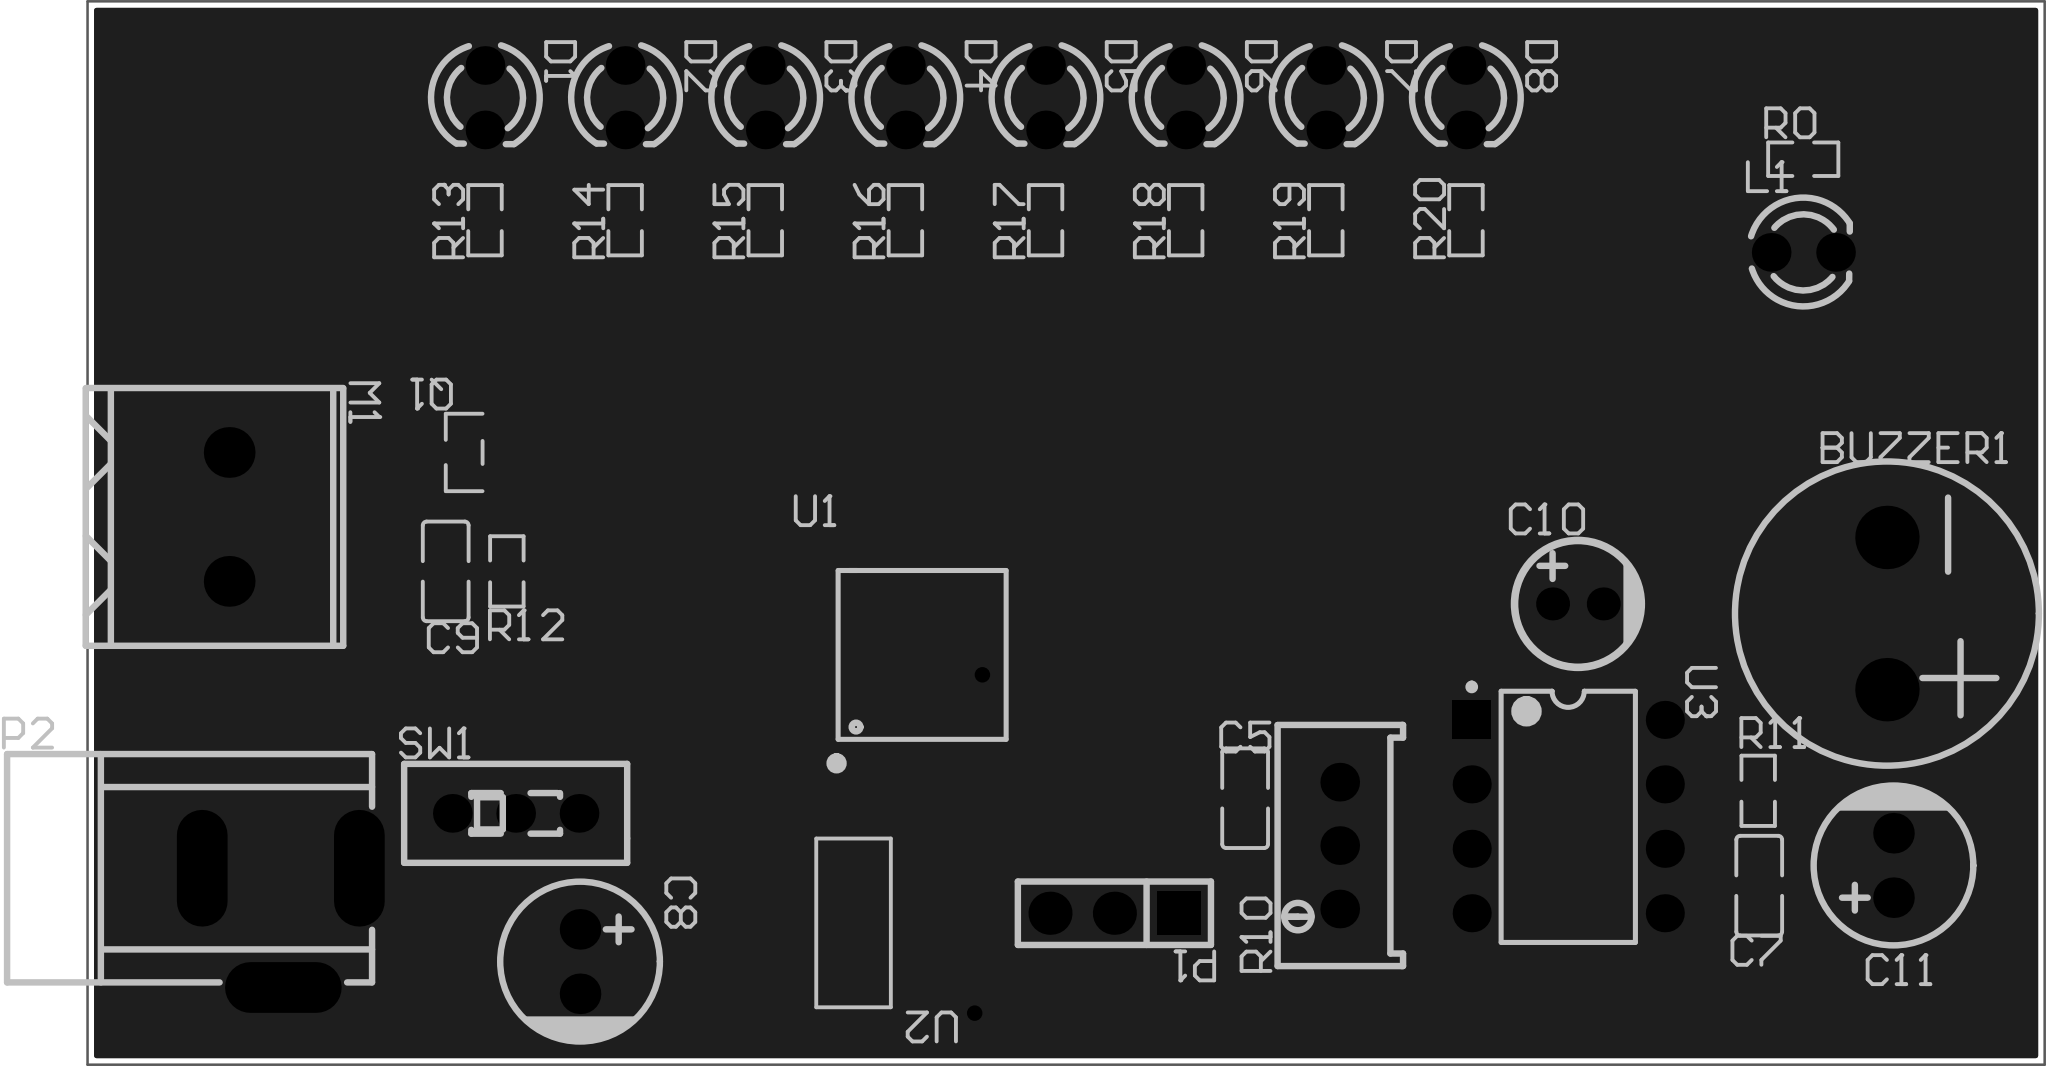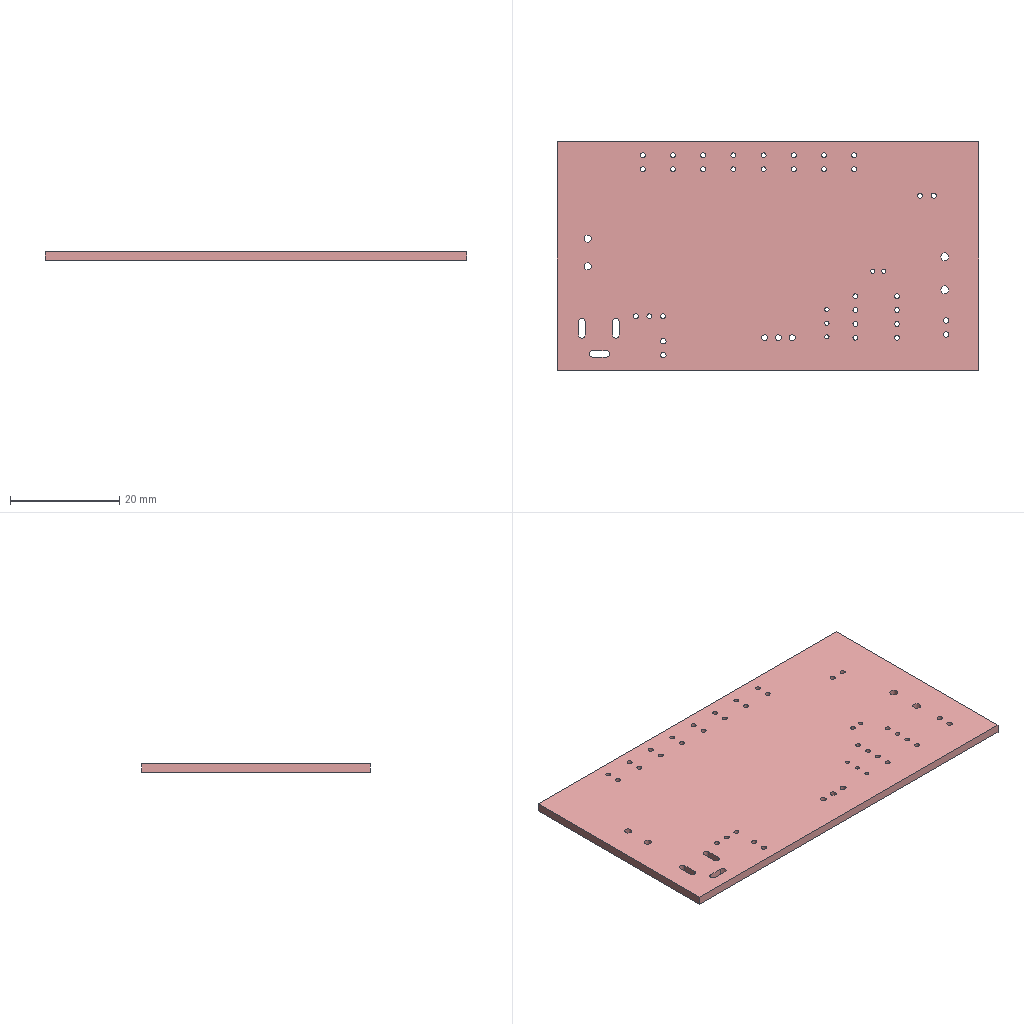Circuit board layout | Altium Designer | box 77.2 x 41.9 x 1.6 mm
Layer stack:
# Altium Designer layer stack of  (unit mm; dielectric type: 0 none, 1 core, 2 prepreg, 3 surface material)
index,name,kind,layer,copper_thickness_mm,dielectric_type,dielectric_thickness_mm,dielectric_material,dielectric_constant
0,Top Paste Mask Layer,other,,,,,,
1,Top Silkscreen Layer,other,,,,,,
2,Top Solder Mask Layer,dielectric,,,3,0.01,,3.3
3,Top Layer,copper,Top Layer,0.035,,,,
4,Dielectric1,dielectric,,,3,1.51,FR4,4.5
5,Bottom Layer,copper,Bottom Layer,0.035,,,,
6,Bottom Solder Mask Layer,dielectric,,,3,0.01,,3.3
7,Bottom Silkscreen Layer,other,,,,,,
8,Bottom Paste Mask Layer,other,,,,,,
# drill layer pairs: low layer,high layer
drill_pair,Top Layer,Bottom Layer
Part placement:
Designator,Comment,Layer,Footprint,Center-X(mm),Center-Y(mm),Rotation
BUZZER1,buzzer,TopLayer,BUZ-TH_BD12.0-P6.00-D0.9-RD,150.368,96.647,270
C5,104,TopLayer,C0805,125.046,89.37,270
C7,104,TopLayer,C0805,145.329,85.924,90
C8,220uF,TopLayer,CAP-TH_BD6.3-P2.50-D1.0-FD,98.806,82.931,270
C9,104,TopLayer,C0805,93.505,98.31,90
C10,10uF,TopLayer,CAP-TH_BD5.0-P2.00-D0.8-FD,138.176,97.028,0
C11,220uF,TopLayer,CAP-TH_BD6.3-P2.50-D1.0-FD,150.626,86.719,90
D1,LED0,TopLayer,LED_TH-3mm,95.055,116.978,270
D2,LED0,TopLayer,LED_TH-3mm,100.585,116.978,270
D3,LED0,TopLayer,LED_TH-3mm,106.114,116.978,270
D4,LED0,TopLayer,LED_TH-3mm,111.643,116.978,270
D5,LED0,TopLayer,LED_TH-3mm,117.172,116.978,270
D6,LED0,TopLayer,LED_TH-3mm,122.701,116.978,270
D7,LED0,TopLayer,LED_TH-3mm,128.23,116.978,270
D8,LED0,TopLayer,LED_TH-3mm,133.759,116.978,270
L1,RED,TopLayer,LED_TH-3mm,147.071,110.882,0
M1,Motor,TopLayer,CONN-TH_2P-P5.08-WJ500V-5.08-2P,84.963,100.457,270
P1,,TopLayer,HDR-TH_3P-P2.54-V-M,119.888,84.836,180
P2,DC005,TopLayer,DC-IN-TH_DC005,87,84.26,0
Q1,9012,TopLayer,SOT-23-3_L2.9-W1.3-P1.90-LS2.4-BR,94.234,102.997,0
R0,1K,TopLayer,R0603,147.066,114.554,0
R10,10kΩ,TopLayer,R_3296,128.778,87.503,90
R11,4.7,TopLayer,R0603,145.288,89.662,270
R12,1K,TopLayer,R0603,95.918,98.31,270
R13,1K,TopLayer,R0603,95.055,112.15,90
R14,1K,TopLayer,R0603,100.585,112.15,90
R15,1K,TopLayer,R0603,106.114,112.15,90
R16,1K,TopLayer,R0603,111.643,112.15,90
R17,1K,TopLayer,R0603,117.172,112.15,90
R18,1K,TopLayer,R0603,122.701,112.15,90
R19,1K,TopLayer,R0603,128.23,112.15,90
R20,1K,TopLayer,R0603,133.759,112.15,90
SW1,Switch,TopLayer,SW-TH_SS-12D01-GX,96.266,88.773,0
U1,STM32F103,TopLayer,LQFP-48_L7.0-W7.0-P0.50-LS9.0-BL,112.315,95.005,0
U2,AMS1117,TopLayer,SOT-223-3_L6.5-W3.4-P2.30-LS7.0-BR,109.497,84.455,180
U3,LM386N-3/NOPB,TopLayer,DIP-8_L9.8-W6.6-P2.54-LS7.6-BL,137.795,88.646,270
Pad and via stacks:
# Altium Designer via and pad stacks of  (unit mm). Each distinct definition once, with the count of objects using it.
# via: kind,start_layer,end_layer,hole_mm,diameter_mm,mode(0 simple;1 top-mid-bottom;2 full stack),diameter_per_layer,count,example_net
# pad: kind,layer,hole_mm,hole_type(0 round;1 square;2 slot),plating,top_size,top_shape(1 round;2 rect;3 octagon;9 rounded rect),mid_size,bottom_size,mode,footprint,size_per_layer,count,example
pad,Multi-Layer,1.5,0,plated,2.5x2.5,1,2.5x2.5,2.5x2.5,0,BUZ-TH_BD12.0-P6.00-D0.9-RD,,2,BUZZER1.1
pad,Multi-Layer,1,0,plated,1.6x1.6,1,1.6x1.6,1.6x1.6,0,CAP-TH_BD6.3-P2.50-D1.0-FD,,4,C8.1
pad,Multi-Layer,0.8,0,plated,1.3x1.3,1,1.3x1.3,1.3x1.3,0,CAP-TH_BD5.0-P2.00-D0.8-FD,,2,C10.1
pad,Multi-Layer,0.9144,0,plated,1.524x1.524,1,1.524x1.524,1.524x1.524,0,LED_TH-3mm,,18,D1.1
pad,Multi-Layer,1.3,0,plated,2x2,1,2x2,2x2,0,CONN-TH_2P-P5.08-WJ500V-5.08-2P,,2,M1.2
pad,Multi-Layer,1.1,0,plated,1.7x1.7,2,1.7x1.7,1.7x1.7,0,HDR-TH_3P-P2.54-V-M,,1,P1.1
pad,Multi-Layer,1.1,0,plated,1.7x1.7,1,1.7x1.7,1.7x1.7,0,HDR-TH_3P-P2.54-V-M,,2,P1.2
pad,Multi-Layer,1.2,2,plated,2x4.6,1,2x4.6,2x4.6,0,DC-IN-TH_DC005,,2,P2.1
pad,Multi-Layer,1.2,2,plated,4.6x2,1,4.6x2,4.6x2,0,DC-IN-TH_DC005,,1,P2.3
pad,Multi-Layer,0.762,0,plated,1.524x1.524,1,1.524x1.524,1.524x1.524,0,R_3296,,3,R10.2
pad,Multi-Layer,0.9144,0,plated,1.524x1.524,1,1.524x1.524,1.524x1.524,0,SW-TH_SS-12D01-GX,,3,SW1.1
pad,Multi-Layer,0.9,0,plated,1.5x1.5,2,1.5x1.5,1.5x1.5,0,DIP-8_L9.8-W6.6-P2.54-LS7.6-BL,,1,U3.1
pad,Multi-Layer,0.9,0,plated,1.5x1.5,1,1.5x1.5,1.5x1.5,0,DIP-8_L9.8-W6.6-P2.54-LS7.6-BL,,7,U3.2
pad,Top Layer,0,0,plated,1.41x1.35,2,1.41x1.35,1.41x1.35,0,C0805,,6,C5.2
pad,Top Layer,0,0,plated,1.25x0.7,2,1.25x0.7,1.25x0.7,0,SOT-23-3_L2.9-W1.3-P1.90-LS2.4-BR,,3,Q1.1
pad,Top Layer,0,0,plated,0.8065x0.864,2,0.8065x0.864,0.8065x0.864,0,R0603,,22,R0.2
pad,Top Layer,0,0,plated,0.27x1.5,1,0.27x1.5,0.27x1.5,0,LQFP-48_L7.0-W7.0-P0.50-LS9.0-BL,,24,U1.1
pad,Top Layer,0,0,plated,1.5x0.27,1,1.5x0.27,1.5x0.27,0,LQFP-48_L7.0-W7.0-P0.50-LS9.0-BL,,24,U1.13
pad,Top Layer,0,0,plated,2.5x1.1,2,2.5x1.1,2.5x1.1,0,SOT-223-3_L6.5-W3.4-P2.30-LS7.0-BR,,3,U2.1
pad,Top Layer,0,0,plated,2.34x3.6,2,2.34x3.6,2.34x3.6,0,SOT-223-3_L6.5-W3.4-P2.30-LS7.0-BR,,1,U2.4
via,Top Layer,Bottom Layer,0.3048,0.6096,0,,2,VCC
Copper pours:
name,layer,net,type(0 solid;1 hatched;2 none)
Top Layer-GND,Top Layer,GND,0
Bottom Layer-GND,Bottom Layer,GND,0